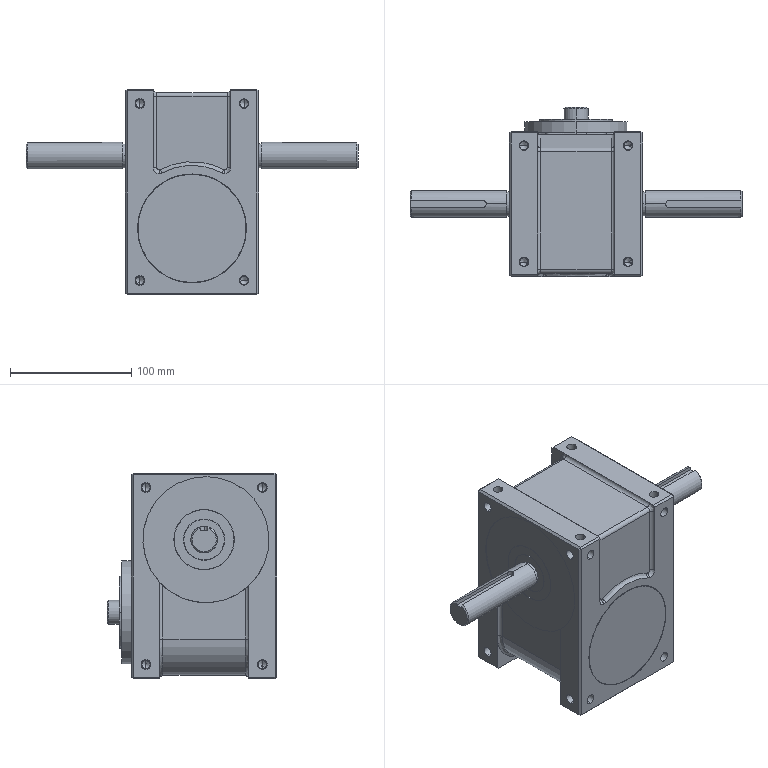Part | SolidWorks | features BaseBody 1 | 1 solid | 825 faces | box 274 x 140 x 170 mm | volume 2182466 mm3 | cylinder 399 | plane 298 | cone 97 | spline 31 | commonest cylinder face diameters 8 x240 6.8 x48 5 x24 1 x22 6 x20 104 x9